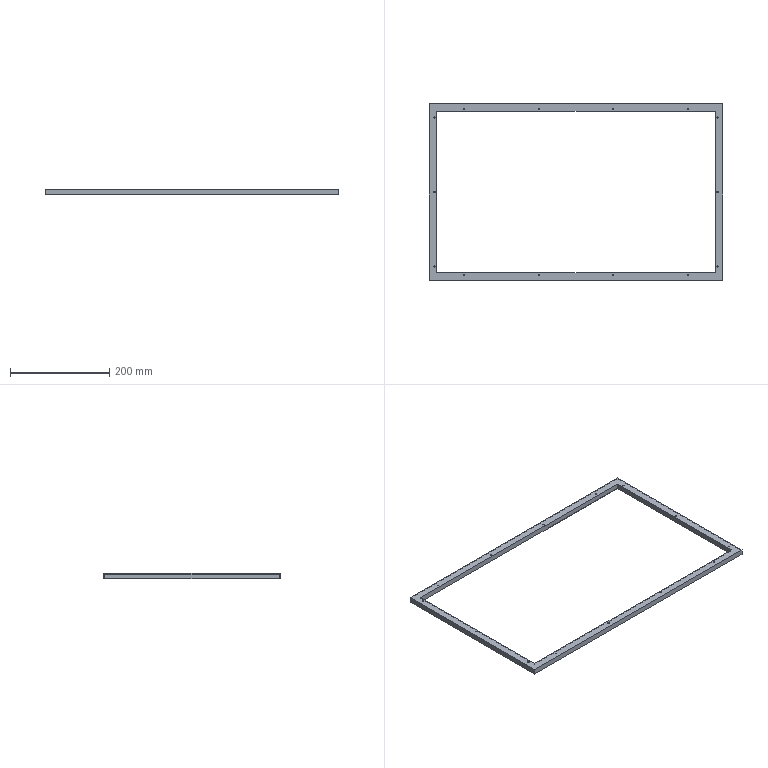Part | STEP file | Glass mouth reinforcing frame 001 | 1 solid | 48 faces | box 590 x 355 x 11 mm | volume 93227 mm3 | cylinder 28 | plane 20 | commonest cylinder face diameters 2.5 x28